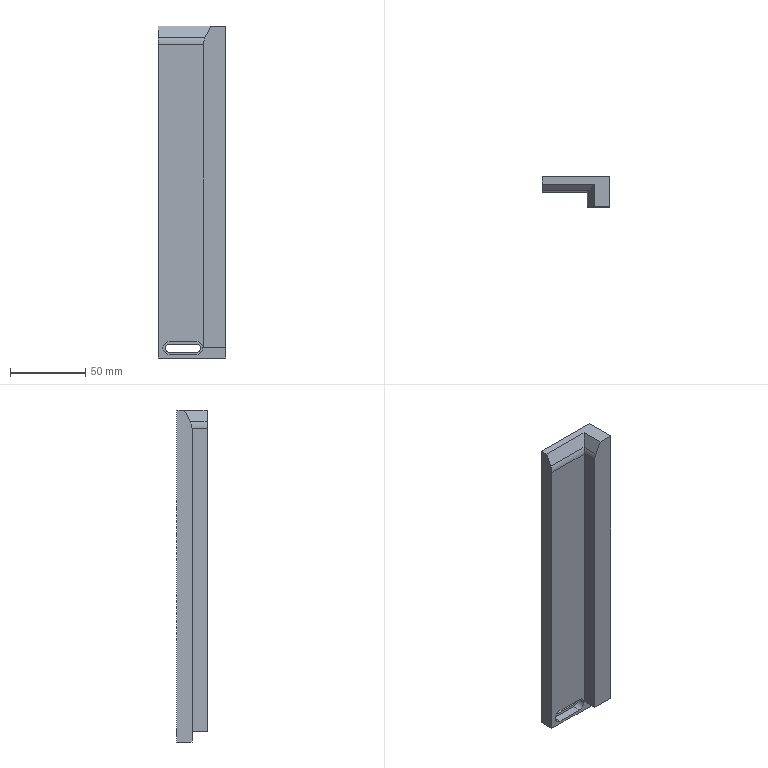Part | STEP file | Tube feed_id566_x_t | 1 solid | 22 faces | box 45 x 20 x 220 mm | volume 128179 mm3 | plane 16 | cylinder 6 | commonest cylinder face diameters 5.2 x2 8.5 x2 20 x2